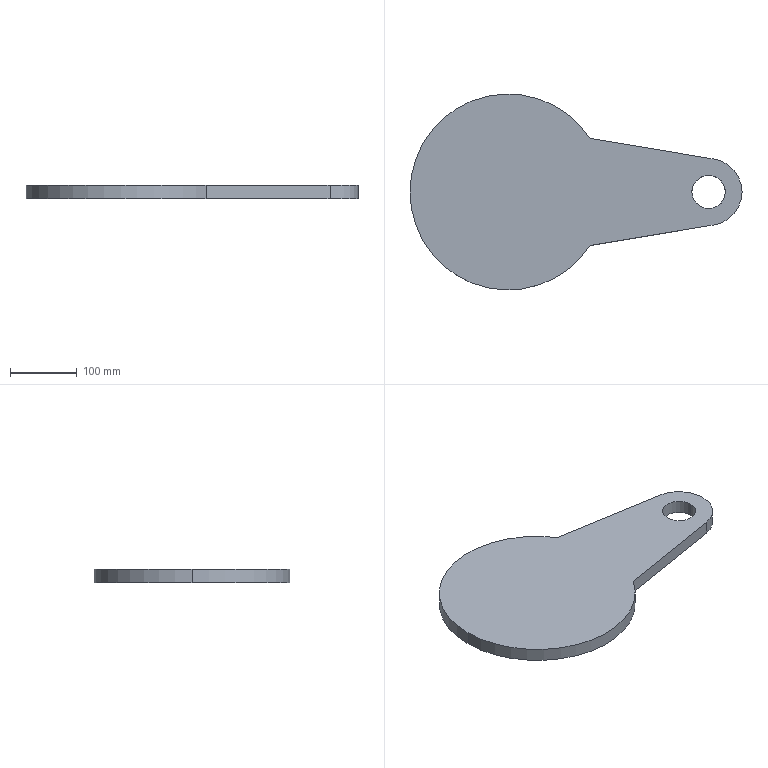Part | SolidWorks | features Extrusion 1 | 1 solid | 9 faces | box 496.5 x 293 x 20 mm | volume 1799574 mm3 | cylinder 5 | plane 4 | commonest cylinder face diameters 50 x2 293 x2 100 x1
STEP:
#1=CARTESIAN_POINT('',(275.,0.,20.));
#2=VERTEX_POINT('',#1);
#3=CARTESIAN_POINT('',(325.,0.,20.));
#4=VERTEX_POINT('',#3);
#5=CARTESIAN_POINT('',(300.,0.,20.));
#6=DIRECTION('',(0.,0.,1.));
#7=DIRECTION('',(1.,0.,0.));
#8=AXIS2_PLACEMENT_3D('',#5,#6,#7);
#9=CIRCLE('',#8,25.);
#10=EDGE_CURVE('',#2,#4,#9,.T.);
#11=ORIENTED_EDGE('',*,*,#10,.T.);
#12=CARTESIAN_POINT('',(325.,0.,0.));
#13=VERTEX_POINT('',#12);
#14=CARTESIAN_POINT('',(325.,0.,20.));
#15=DIRECTION('',(0.,0.,-1.));
#16=VECTOR('',#15,1000.);
#17=LINE('',#14,#16);
#18=EDGE_CURVE('',#4,#13,#17,.T.);
#19=ORIENTED_EDGE('',*,*,#18,.T.);
#20=CARTESIAN_POINT('',(275.,0.,0.));
#21=VERTEX_POINT('',#20);
#22=CARTESIAN_POINT('',(300.,0.,0.));
#23=DIRECTION('',(0.,0.,1.));
#24=DIRECTION('',(1.,0.,0.));
#25=AXIS2_PLACEMENT_3D('',#22,#23,#24);
#26=CIRCLE('',#25,25.);
#27=EDGE_CURVE('',#21,#13,#26,.T.);
#28=ORIENTED_EDGE('',*,*,#27,.F.);
#29=CARTESIAN_POINT('',(275.,0.,20.));
#30=DIRECTION('',(0.,0.,-1.));
#31=VECTOR('',#30,1000.);
#32=LINE('',#29,#31);
#33=EDGE_CURVE('',#2,#21,#32,.T.);
#34=ORIENTED_EDGE('',*,*,#33,.F.);
#35=EDGE_LOOP('',(#11,#19,#28,#34));
#36=FACE_OUTER_BOUND('',#35,.T.);
#37=CARTESIAN_POINT('',(300.,0.,20.));
#38=DIRECTION('',(0.,0.,-1.));
#39=DIRECTION('',(-1.,0.,0.));
#40=AXIS2_PLACEMENT_3D('',#37,#38,#39);
#41=CYLINDRICAL_SURFACE('',#40,25.);
#42=ADVANCED_FACE('',(#36),#41,.F.);
#43=CARTESIAN_POINT('',(-146.5,0.,20.));
#44=VERTEX_POINT('',#43);
#45=CARTESIAN_POINT('',(122.728,-80.,20.));
#46=VERTEX_POINT('',#45);
#47=CARTESIAN_POINT('',(0.,0.,20.));
#48=DIRECTION('',(0.,0.,1.));
#49=DIRECTION('',(1.,0.,0.));
#50=AXIS2_PLACEMENT_3D('',#47,#48,#49);
#51=CIRCLE('',#50,146.5);
#52=EDGE_CURVE('',#44,#46,#51,.T.);
#53=ORIENTED_EDGE('',*,*,#52,.F.);
#54=CARTESIAN_POINT('',(-146.5,0.,0.));
#55=VERTEX_POINT('',#54);
#56=CARTESIAN_POINT('',(-146.5,0.,20.));
#57=DIRECTION('',(0.,0.,-1.));
#58=VECTOR('',#57,1000.);
#59=LINE('',#56,#58);
#60=EDGE_CURVE('',#44,#55,#59,.T.);
#61=ORIENTED_EDGE('',*,*,#60,.T.);
#62=CARTESIAN_POINT('',(122.728,-80.,0.));
#63=VERTEX_POINT('',#62);
#64=CARTESIAN_POINT('',(0.,0.,0.));
#65=DIRECTION('',(0.,0.,1.));
#66=DIRECTION('',(1.,0.,0.));
#67=AXIS2_PLACEMENT_3D('',#64,#65,#66);
#68=CIRCLE('',#67,146.5);
#69=EDGE_CURVE('',#55,#63,#68,.T.);
#70=ORIENTED_EDGE('',*,*,#69,.T.);
#71=CARTESIAN_POINT('',(122.728,-80.,20.));
#72=DIRECTION('',(0.,0.,-1.));
#73=VECTOR('',#72,1000.);
#74=LINE('',#71,#73);
#75=EDGE_CURVE('',#46,#63,#74,.T.);
#76=ORIENTED_EDGE('',*,*,#75,.F.);
#77=EDGE_LOOP('',(#53,#61,#70,#76));
#78=FACE_OUTER_BOUND('',#77,.T.);
#79=CARTESIAN_POINT('',(0.,0.,20.));
#80=DIRECTION('',(0.,0.,-1.));
#81=DIRECTION('',(-1.,0.,0.));
#82=AXIS2_PLACEMENT_3D('',#79,#80,#81);
#83=CYLINDRICAL_SURFACE('',#82,146.5);
#84=ADVANCED_FACE('',(#78),#83,.T.);
#85=CARTESIAN_POINT('',(122.728,80.,20.));
#86=VERTEX_POINT('',#85);
#87=CARTESIAN_POINT('',(0.,0.,20.));
#88=DIRECTION('',(0.,0.,1.));
#89=DIRECTION('',(1.,0.,0.));
#90=AXIS2_PLACEMENT_3D('',#87,#88,#89);
#91=CIRCLE('',#90,146.5);
#92=EDGE_CURVE('',#86,#44,#91,.T.);
#93=ORIENTED_EDGE('',*,*,#92,.T.);
#94=ORIENTED_EDGE('',*,*,#52,.T.);
#95=CARTESIAN_POINT('',(308.159,-49.33,20.));
#96=VERTEX_POINT('',#95);
#97=CARTESIAN_POINT('',(122.728,-80.,20.));
#98=DIRECTION('',(0.9866,0.1632,0.));
#99=VECTOR('',#98,1000.);
#100=LINE('',#97,#99);
#101=EDGE_CURVE('',#46,#96,#100,.T.);
#102=ORIENTED_EDGE('',*,*,#101,.T.);
#103=CARTESIAN_POINT('',(308.159,49.33,20.));
#104=VERTEX_POINT('',#103);
#105=CARTESIAN_POINT('',(300.,0.,20.));
#106=DIRECTION('',(0.,0.,1.));
#107=DIRECTION('',(1.,0.,0.));
#108=AXIS2_PLACEMENT_3D('',#105,#106,#107);
#109=CIRCLE('',#108,50.);
#110=EDGE_CURVE('',#96,#104,#109,.T.);
#111=ORIENTED_EDGE('',*,*,#110,.T.);
#112=CARTESIAN_POINT('',(122.728,80.,20.));
#113=DIRECTION('',(-0.9866,0.1632,0.));
#114=VECTOR('',#113,1000.);
#115=LINE('',#112,#114);
#116=EDGE_CURVE('',#104,#86,#115,.T.);
#117=ORIENTED_EDGE('',*,*,#116,.T.);
#118=EDGE_LOOP('',(#93,#94,#102,#111,#117));
#119=FACE_OUTER_BOUND('',#118,.T.);
#120=ORIENTED_EDGE('',*,*,#10,.F.);
#121=CARTESIAN_POINT('',(300.,0.,20.));
#122=DIRECTION('',(0.,0.,1.));
#123=DIRECTION('',(1.,0.,0.));
#124=AXIS2_PLACEMENT_3D('',#121,#122,#123);
#125=CIRCLE('',#124,25.);
#126=EDGE_CURVE('',#4,#2,#125,.T.);
#127=ORIENTED_EDGE('',*,*,#126,.F.);
#128=EDGE_LOOP('',(#120,#127));
#129=FACE_BOUND('',#128,.T.);
#130=CARTESIAN_POINT('',(0.,0.,20.));
#131=DIRECTION('',(0.,0.,1.));
#132=DIRECTION('',(1.,0.,0.));
#133=AXIS2_PLACEMENT_3D('',#130,#131,#132);
#134=PLANE('',#133);
#135=ADVANCED_FACE('',(#119,#129),#134,.T.);
#136=CARTESIAN_POINT('',(122.728,80.,0.));
#137=VERTEX_POINT('',#136);
#138=CARTESIAN_POINT('',(0.,0.,0.));
#139=DIRECTION('',(0.,0.,1.));
#140=DIRECTION('',(1.,0.,0.));
#141=AXIS2_PLACEMENT_3D('',#138,#139,#140);
#142=CIRCLE('',#141,146.5);
#143=EDGE_CURVE('',#137,#55,#142,.T.);
#144=ORIENTED_EDGE('',*,*,#143,.F.);
#145=CARTESIAN_POINT('',(308.159,49.33,0.));
#146=VERTEX_POINT('',#145);
#147=CARTESIAN_POINT('',(122.728,80.,0.));
#148=DIRECTION('',(-0.9866,0.1632,0.));
#149=VECTOR('',#148,1000.);
#150=LINE('',#147,#149);
#151=EDGE_CURVE('',#146,#137,#150,.T.);
#152=ORIENTED_EDGE('',*,*,#151,.F.);
#153=CARTESIAN_POINT('',(308.159,-49.33,0.));
#154=VERTEX_POINT('',#153);
#155=CARTESIAN_POINT('',(300.,0.,0.));
#156=DIRECTION('',(0.,0.,1.));
#157=DIRECTION('',(1.,0.,0.));
#158=AXIS2_PLACEMENT_3D('',#155,#156,#157);
#159=CIRCLE('',#158,50.);
#160=EDGE_CURVE('',#154,#146,#159,.T.);
#161=ORIENTED_EDGE('',*,*,#160,.F.);
#162=CARTESIAN_POINT('',(122.728,-80.,0.));
#163=DIRECTION('',(0.9866,0.1632,0.));
#164=VECTOR('',#163,1000.);
#165=LINE('',#162,#164);
#166=EDGE_CURVE('',#63,#154,#165,.T.);
#167=ORIENTED_EDGE('',*,*,#166,.F.);
#168=ORIENTED_EDGE('',*,*,#69,.F.);
#169=EDGE_LOOP('',(#144,#152,#161,#167,#168));
#170=FACE_OUTER_BOUND('',#169,.T.);
#171=ORIENTED_EDGE('',*,*,#27,.T.);
#172=CARTESIAN_POINT('',(300.,0.,0.));
#173=DIRECTION('',(0.,0.,1.));
#174=DIRECTION('',(1.,0.,0.));
#175=AXIS2_PLACEMENT_3D('',#172,#173,#174);
#176=CIRCLE('',#175,25.);
#177=EDGE_CURVE('',#13,#21,#176,.T.);
#178=ORIENTED_EDGE('',*,*,#177,.T.);
#179=EDGE_LOOP('',(#171,#178));
#180=FACE_BOUND('',#179,.T.);
#181=CARTESIAN_POINT('',(0.,0.,0.));
#182=DIRECTION('',(0.,0.,1.));
#183=DIRECTION('',(1.,0.,0.));
#184=AXIS2_PLACEMENT_3D('',#181,#182,#183);
#185=PLANE('',#184);
#186=ADVANCED_FACE('',(#170,#180),#185,.F.);
#187=ORIENTED_EDGE('',*,*,#60,.F.);
#188=ORIENTED_EDGE('',*,*,#92,.F.);
#189=CARTESIAN_POINT('',(122.728,80.,20.));
#190=DIRECTION('',(0.,0.,-1.));
#191=VECTOR('',#190,1000.);
#192=LINE('',#189,#191);
#193=EDGE_CURVE('',#86,#137,#192,.T.);
#194=ORIENTED_EDGE('',*,*,#193,.T.);
#195=ORIENTED_EDGE('',*,*,#143,.T.);
#196=EDGE_LOOP('',(#187,#188,#194,#195));
#197=FACE_OUTER_BOUND('',#196,.T.);
#198=CARTESIAN_POINT('',(0.,0.,20.));
#199=DIRECTION('',(0.,0.,-1.));
#200=DIRECTION('',(-1.,0.,0.));
#201=AXIS2_PLACEMENT_3D('',#198,#199,#200);
#202=CYLINDRICAL_SURFACE('',#201,146.5);
#203=ADVANCED_FACE('',(#197),#202,.T.);
#204=ORIENTED_EDGE('',*,*,#166,.T.);
#205=CARTESIAN_POINT('',(308.159,-49.33,20.));
#206=DIRECTION('',(0.,0.,-1.));
#207=VECTOR('',#206,1000.);
#208=LINE('',#205,#207);
#209=EDGE_CURVE('',#96,#154,#208,.T.);
#210=ORIENTED_EDGE('',*,*,#209,.F.);
#211=ORIENTED_EDGE('',*,*,#101,.F.);
#212=ORIENTED_EDGE('',*,*,#75,.T.);
#213=EDGE_LOOP('',(#204,#210,#211,#212));
#214=FACE_OUTER_BOUND('',#213,.T.);
#215=CARTESIAN_POINT('',(122.728,-80.,20.));
#216=DIRECTION('',(-0.1632,0.9866,0.));
#217=DIRECTION('',(-0.9866,-0.1632,0.));
#218=AXIS2_PLACEMENT_3D('',#215,#216,#217);
#219=PLANE('',#218);
#220=ADVANCED_FACE('',(#214),#219,.F.);
#221=ORIENTED_EDGE('',*,*,#160,.T.);
#222=CARTESIAN_POINT('',(308.159,49.33,20.));
#223=DIRECTION('',(0.,0.,-1.));
#224=VECTOR('',#223,1000.);
#225=LINE('',#222,#224);
#226=EDGE_CURVE('',#104,#146,#225,.T.);
#227=ORIENTED_EDGE('',*,*,#226,.F.);
#228=ORIENTED_EDGE('',*,*,#110,.F.);
#229=ORIENTED_EDGE('',*,*,#209,.T.);
#230=EDGE_LOOP('',(#221,#227,#228,#229));
#231=FACE_OUTER_BOUND('',#230,.T.);
#232=CARTESIAN_POINT('',(300.,0.,20.));
#233=DIRECTION('',(0.,0.,-1.));
#234=DIRECTION('',(-1.,0.,0.));
#235=AXIS2_PLACEMENT_3D('',#232,#233,#234);
#236=CYLINDRICAL_SURFACE('',#235,50.);
#237=ADVANCED_FACE('',(#231),#236,.T.);
#238=ORIENTED_EDGE('',*,*,#151,.T.);
#239=ORIENTED_EDGE('',*,*,#193,.F.);
#240=ORIENTED_EDGE('',*,*,#116,.F.);
#241=ORIENTED_EDGE('',*,*,#226,.T.);
#242=EDGE_LOOP('',(#238,#239,#240,#241));
#243=FACE_OUTER_BOUND('',#242,.T.);
#244=CARTESIAN_POINT('',(122.728,80.,20.));
#245=DIRECTION('',(-0.1632,-0.9866,0.));
#246=DIRECTION('',(0.9866,-0.1632,0.));
#247=AXIS2_PLACEMENT_3D('',#244,#245,#246);
#248=PLANE('',#247);
#249=ADVANCED_FACE('',(#243),#248,.F.);
#250=ORIENTED_EDGE('',*,*,#18,.F.);
#251=ORIENTED_EDGE('',*,*,#126,.T.);
#252=ORIENTED_EDGE('',*,*,#33,.T.);
#253=ORIENTED_EDGE('',*,*,#177,.F.);
#254=EDGE_LOOP('',(#250,#251,#252,#253));
#255=FACE_OUTER_BOUND('',#254,.T.);
#256=CARTESIAN_POINT('',(300.,0.,20.));
#257=DIRECTION('',(0.,0.,-1.));
#258=DIRECTION('',(-1.,0.,0.));
#259=AXIS2_PLACEMENT_3D('',#256,#257,#258);
#260=CYLINDRICAL_SURFACE('',#259,25.);
#261=ADVANCED_FACE('',(#255),#260,.F.);
#262=CLOSED_SHELL('',(#42,#84,#135,#186,#203,#220,#237,#249,#261));
#263=MANIFOLD_SOLID_BREP('',#262);
#264=CARTESIAN_POINT('',(0.,0.,0.));
#265=DIRECTION('',(0.,0.,1.));
#266=DIRECTION('',(1.,0.,0.));
#267=AXIS2_PLACEMENT_3D('',#264,#265,#266);
#268=(LENGTH_UNIT()NAMED_UNIT(*)SI_UNIT(.MILLI.,.METRE.));
#269=UNCERTAINTY_MEASURE_WITH_UNIT(LENGTH_MEASURE(0.00001),#268,'','');
#270=(NAMED_UNIT(*)PLANE_ANGLE_UNIT()SI_UNIT($,.RADIAN.));
#271=(NAMED_UNIT(*)SI_UNIT($,.STERADIAN.)SOLID_ANGLE_UNIT());
#272=(GEOMETRIC_REPRESENTATION_CONTEXT(3)GLOBAL_UNCERTAINTY_ASSIGNED_CONTEXT((#269))GLOBAL_UNIT_ASSIGNED_CONTEXT((#268,#270,#271))REPRESENTATION_CONTEXT('',''));
#273=ADVANCED_BREP_SHAPE_REPRESENTATION('',(#263,#267),#272);